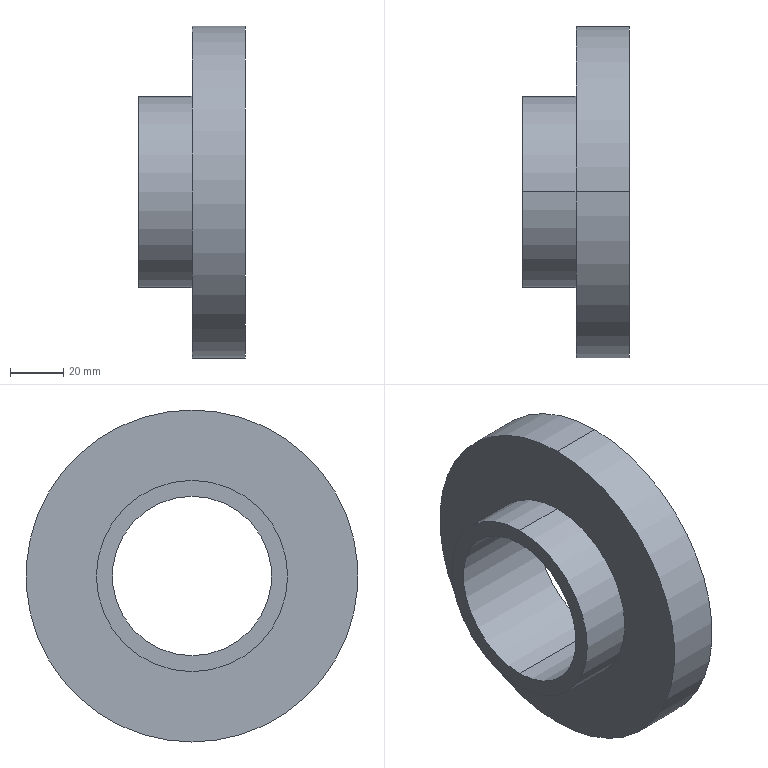Part | SolidWorks | features Revolution 1 | 1 solid | 9 faces | box 40 x 125 x 125 mm | volume 213770 mm3 | cylinder 6 | plane 3 | commonest cylinder face diameters 60 x2 72 x2 125 x2
STEP:
#1=CARTESIAN_POINT('',(40.,0.,62.5));
#2=VERTEX_POINT('',#1);
#3=CARTESIAN_POINT('',(40.,0.,-62.5));
#4=VERTEX_POINT('',#3);
#5=CARTESIAN_POINT('',(40.,0.,0.));
#6=DIRECTION('',(-1.,0.,0.));
#7=DIRECTION('',(0.,0.,1.));
#8=AXIS2_PLACEMENT_3D('',#5,#6,#7);
#9=CIRCLE('',#8,62.5);
#10=EDGE_CURVE('',#2,#4,#9,.T.);
#11=ORIENTED_EDGE('',*,*,#10,.T.);
#12=CARTESIAN_POINT('',(20.,0.,-62.5));
#13=VERTEX_POINT('',#12);
#14=CARTESIAN_POINT('',(0.,0.,-62.5));
#15=DIRECTION('',(-1.,0.,0.));
#16=VECTOR('',#15,1000.);
#17=LINE('',#14,#16);
#18=EDGE_CURVE('',#4,#13,#17,.T.);
#19=ORIENTED_EDGE('',*,*,#18,.T.);
#20=CARTESIAN_POINT('',(20.,0.,62.5));
#21=VERTEX_POINT('',#20);
#22=CARTESIAN_POINT('',(20.,0.,0.));
#23=DIRECTION('',(-1.,0.,0.));
#24=DIRECTION('',(0.,0.,1.));
#25=AXIS2_PLACEMENT_3D('',#22,#23,#24);
#26=CIRCLE('',#25,62.5);
#27=EDGE_CURVE('',#21,#13,#26,.T.);
#28=ORIENTED_EDGE('',*,*,#27,.F.);
#29=CARTESIAN_POINT('',(0.,0.,62.5));
#30=DIRECTION('',(-1.,0.,0.));
#31=VECTOR('',#30,1000.);
#32=LINE('',#29,#31);
#33=EDGE_CURVE('',#2,#21,#32,.T.);
#34=ORIENTED_EDGE('',*,*,#33,.F.);
#35=EDGE_LOOP('',(#11,#19,#28,#34));
#36=FACE_OUTER_BOUND('',#35,.T.);
#37=CARTESIAN_POINT('',(0.,0.,0.));
#38=DIRECTION('',(-1.,0.,0.));
#39=DIRECTION('',(0.,0.,1.));
#40=AXIS2_PLACEMENT_3D('',#37,#38,#39);
#41=CYLINDRICAL_SURFACE('',#40,62.5);
#42=ADVANCED_FACE('',(#36),#41,.T.);
#43=CARTESIAN_POINT('',(20.,0.,36.));
#44=VERTEX_POINT('',#43);
#45=CARTESIAN_POINT('',(20.,0.,-36.));
#46=VERTEX_POINT('',#45);
#47=CARTESIAN_POINT('',(20.,0.,0.));
#48=DIRECTION('',(-1.,0.,0.));
#49=DIRECTION('',(0.,0.,1.));
#50=AXIS2_PLACEMENT_3D('',#47,#48,#49);
#51=CIRCLE('',#50,36.);
#52=EDGE_CURVE('',#44,#46,#51,.T.);
#53=ORIENTED_EDGE('',*,*,#52,.T.);
#54=CARTESIAN_POINT('',(0.,0.,-36.));
#55=VERTEX_POINT('',#54);
#56=CARTESIAN_POINT('',(0.,0.,-36.));
#57=DIRECTION('',(-1.,0.,0.));
#58=VECTOR('',#57,1000.);
#59=LINE('',#56,#58);
#60=EDGE_CURVE('',#46,#55,#59,.T.);
#61=ORIENTED_EDGE('',*,*,#60,.T.);
#62=CARTESIAN_POINT('',(0.,0.,36.));
#63=VERTEX_POINT('',#62);
#64=CARTESIAN_POINT('',(0.,0.,0.));
#65=DIRECTION('',(-1.,0.,0.));
#66=DIRECTION('',(0.,0.,1.));
#67=AXIS2_PLACEMENT_3D('',#64,#65,#66);
#68=CIRCLE('',#67,36.);
#69=EDGE_CURVE('',#63,#55,#68,.T.);
#70=ORIENTED_EDGE('',*,*,#69,.F.);
#71=CARTESIAN_POINT('',(0.,0.,36.));
#72=DIRECTION('',(-1.,0.,0.));
#73=VECTOR('',#72,1000.);
#74=LINE('',#71,#73);
#75=EDGE_CURVE('',#44,#63,#74,.T.);
#76=ORIENTED_EDGE('',*,*,#75,.F.);
#77=EDGE_LOOP('',(#53,#61,#70,#76));
#78=FACE_OUTER_BOUND('',#77,.T.);
#79=CARTESIAN_POINT('',(0.,0.,0.));
#80=DIRECTION('',(-1.,0.,0.));
#81=DIRECTION('',(0.,0.,1.));
#82=AXIS2_PLACEMENT_3D('',#79,#80,#81);
#83=CYLINDRICAL_SURFACE('',#82,36.);
#84=ADVANCED_FACE('',(#78),#83,.T.);
#85=CARTESIAN_POINT('',(40.,0.,-30.));
#86=VERTEX_POINT('',#85);
#87=CARTESIAN_POINT('',(40.,0.,30.));
#88=VERTEX_POINT('',#87);
#89=CARTESIAN_POINT('',(40.,0.,0.));
#90=DIRECTION('',(-1.,0.,0.));
#91=DIRECTION('',(0.,0.,1.));
#92=AXIS2_PLACEMENT_3D('',#89,#90,#91);
#93=CIRCLE('',#92,30.);
#94=EDGE_CURVE('',#86,#88,#93,.T.);
#95=ORIENTED_EDGE('',*,*,#94,.F.);
#96=CARTESIAN_POINT('',(0.,0.,-30.));
#97=VERTEX_POINT('',#96);
#98=CARTESIAN_POINT('',(0.,0.,-30.));
#99=DIRECTION('',(-1.,0.,0.));
#100=VECTOR('',#99,1000.);
#101=LINE('',#98,#100);
#102=EDGE_CURVE('',#86,#97,#101,.T.);
#103=ORIENTED_EDGE('',*,*,#102,.T.);
#104=CARTESIAN_POINT('',(0.,0.,30.));
#105=VERTEX_POINT('',#104);
#106=CARTESIAN_POINT('',(0.,0.,0.));
#107=DIRECTION('',(-1.,0.,0.));
#108=DIRECTION('',(0.,0.,1.));
#109=AXIS2_PLACEMENT_3D('',#106,#107,#108);
#110=CIRCLE('',#109,30.);
#111=EDGE_CURVE('',#97,#105,#110,.T.);
#112=ORIENTED_EDGE('',*,*,#111,.T.);
#113=CARTESIAN_POINT('',(0.,0.,30.));
#114=DIRECTION('',(-1.,0.,0.));
#115=VECTOR('',#114,1000.);
#116=LINE('',#113,#115);
#117=EDGE_CURVE('',#88,#105,#116,.T.);
#118=ORIENTED_EDGE('',*,*,#117,.F.);
#119=EDGE_LOOP('',(#95,#103,#112,#118));
#120=FACE_OUTER_BOUND('',#119,.T.);
#121=CARTESIAN_POINT('',(0.,0.,0.));
#122=DIRECTION('',(-1.,0.,0.));
#123=DIRECTION('',(0.,0.,1.));
#124=AXIS2_PLACEMENT_3D('',#121,#122,#123);
#125=CYLINDRICAL_SURFACE('',#124,30.);
#126=ADVANCED_FACE('',(#120),#125,.F.);
#127=ORIENTED_EDGE('',*,*,#102,.F.);
#128=CARTESIAN_POINT('',(40.,0.,0.));
#129=DIRECTION('',(-1.,0.,0.));
#130=DIRECTION('',(0.,0.,1.));
#131=AXIS2_PLACEMENT_3D('',#128,#129,#130);
#132=CIRCLE('',#131,30.);
#133=EDGE_CURVE('',#88,#86,#132,.T.);
#134=ORIENTED_EDGE('',*,*,#133,.F.);
#135=ORIENTED_EDGE('',*,*,#117,.T.);
#136=CARTESIAN_POINT('',(0.,0.,0.));
#137=DIRECTION('',(-1.,0.,0.));
#138=DIRECTION('',(0.,0.,1.));
#139=AXIS2_PLACEMENT_3D('',#136,#137,#138);
#140=CIRCLE('',#139,30.);
#141=EDGE_CURVE('',#105,#97,#140,.T.);
#142=ORIENTED_EDGE('',*,*,#141,.T.);
#143=EDGE_LOOP('',(#127,#134,#135,#142));
#144=FACE_OUTER_BOUND('',#143,.T.);
#145=CARTESIAN_POINT('',(0.,0.,0.));
#146=DIRECTION('',(-1.,0.,0.));
#147=DIRECTION('',(0.,0.,1.));
#148=AXIS2_PLACEMENT_3D('',#145,#146,#147);
#149=CYLINDRICAL_SURFACE('',#148,30.);
#150=ADVANCED_FACE('',(#144),#149,.F.);
#151=ORIENTED_EDGE('',*,*,#69,.T.);
#152=CARTESIAN_POINT('',(0.,0.,0.));
#153=DIRECTION('',(-1.,0.,0.));
#154=DIRECTION('',(0.,0.,1.));
#155=AXIS2_PLACEMENT_3D('',#152,#153,#154);
#156=CIRCLE('',#155,36.);
#157=EDGE_CURVE('',#55,#63,#156,.T.);
#158=ORIENTED_EDGE('',*,*,#157,.T.);
#159=EDGE_LOOP('',(#151,#158));
#160=FACE_OUTER_BOUND('',#159,.T.);
#161=ORIENTED_EDGE('',*,*,#141,.F.);
#162=ORIENTED_EDGE('',*,*,#111,.F.);
#163=EDGE_LOOP('',(#161,#162));
#164=FACE_BOUND('',#163,.T.);
#165=CARTESIAN_POINT('',(0.,-30.,0.));
#166=DIRECTION('',(-1.,0.,0.));
#167=DIRECTION('',(0.,0.,1.));
#168=AXIS2_PLACEMENT_3D('',#165,#166,#167);
#169=PLANE('',#168);
#170=ADVANCED_FACE('',(#160,#164),#169,.T.);
#171=ORIENTED_EDGE('',*,*,#60,.F.);
#172=CARTESIAN_POINT('',(20.,0.,0.));
#173=DIRECTION('',(-1.,0.,0.));
#174=DIRECTION('',(0.,0.,1.));
#175=AXIS2_PLACEMENT_3D('',#172,#173,#174);
#176=CIRCLE('',#175,36.);
#177=EDGE_CURVE('',#46,#44,#176,.T.);
#178=ORIENTED_EDGE('',*,*,#177,.T.);
#179=ORIENTED_EDGE('',*,*,#75,.T.);
#180=ORIENTED_EDGE('',*,*,#157,.F.);
#181=EDGE_LOOP('',(#171,#178,#179,#180));
#182=FACE_OUTER_BOUND('',#181,.T.);
#183=CARTESIAN_POINT('',(0.,0.,0.));
#184=DIRECTION('',(-1.,0.,0.));
#185=DIRECTION('',(0.,0.,1.));
#186=AXIS2_PLACEMENT_3D('',#183,#184,#185);
#187=CYLINDRICAL_SURFACE('',#186,36.);
#188=ADVANCED_FACE('',(#182),#187,.T.);
#189=ORIENTED_EDGE('',*,*,#27,.T.);
#190=CARTESIAN_POINT('',(20.,0.,0.));
#191=DIRECTION('',(-1.,0.,0.));
#192=DIRECTION('',(0.,0.,1.));
#193=AXIS2_PLACEMENT_3D('',#190,#191,#192);
#194=CIRCLE('',#193,62.5);
#195=EDGE_CURVE('',#13,#21,#194,.T.);
#196=ORIENTED_EDGE('',*,*,#195,.T.);
#197=EDGE_LOOP('',(#189,#196));
#198=FACE_OUTER_BOUND('',#197,.T.);
#199=ORIENTED_EDGE('',*,*,#52,.F.);
#200=ORIENTED_EDGE('',*,*,#177,.F.);
#201=EDGE_LOOP('',(#199,#200));
#202=FACE_BOUND('',#201,.T.);
#203=CARTESIAN_POINT('',(20.,-36.,0.));
#204=DIRECTION('',(-1.,0.,0.));
#205=DIRECTION('',(0.,0.,1.));
#206=AXIS2_PLACEMENT_3D('',#203,#204,#205);
#207=PLANE('',#206);
#208=ADVANCED_FACE('',(#198,#202),#207,.T.);
#209=ORIENTED_EDGE('',*,*,#18,.F.);
#210=CARTESIAN_POINT('',(40.,0.,0.));
#211=DIRECTION('',(-1.,0.,0.));
#212=DIRECTION('',(0.,0.,1.));
#213=AXIS2_PLACEMENT_3D('',#210,#211,#212);
#214=CIRCLE('',#213,62.5);
#215=EDGE_CURVE('',#4,#2,#214,.T.);
#216=ORIENTED_EDGE('',*,*,#215,.T.);
#217=ORIENTED_EDGE('',*,*,#33,.T.);
#218=ORIENTED_EDGE('',*,*,#195,.F.);
#219=EDGE_LOOP('',(#209,#216,#217,#218));
#220=FACE_OUTER_BOUND('',#219,.T.);
#221=CARTESIAN_POINT('',(0.,0.,0.));
#222=DIRECTION('',(-1.,0.,0.));
#223=DIRECTION('',(0.,0.,1.));
#224=AXIS2_PLACEMENT_3D('',#221,#222,#223);
#225=CYLINDRICAL_SURFACE('',#224,62.5);
#226=ADVANCED_FACE('',(#220),#225,.T.);
#227=ORIENTED_EDGE('',*,*,#133,.T.);
#228=ORIENTED_EDGE('',*,*,#94,.T.);
#229=EDGE_LOOP('',(#227,#228));
#230=FACE_BOUND('',#229,.T.);
#231=ORIENTED_EDGE('',*,*,#10,.F.);
#232=ORIENTED_EDGE('',*,*,#215,.F.);
#233=EDGE_LOOP('',(#231,#232));
#234=FACE_OUTER_BOUND('',#233,.T.);
#235=CARTESIAN_POINT('',(40.,-62.5,0.));
#236=DIRECTION('',(1.,0.,0.));
#237=DIRECTION('',(0.,0.,-1.));
#238=AXIS2_PLACEMENT_3D('',#235,#236,#237);
#239=PLANE('',#238);
#240=ADVANCED_FACE('',(#230,#234),#239,.T.);
#241=CLOSED_SHELL('',(#42,#84,#126,#150,#170,#188,#208,#226,#240));
#242=MANIFOLD_SOLID_BREP('',#241);
#243=CARTESIAN_POINT('',(0.,0.,0.));
#244=DIRECTION('',(0.,0.,1.));
#245=DIRECTION('',(1.,0.,0.));
#246=AXIS2_PLACEMENT_3D('',#243,#244,#245);
#247=(LENGTH_UNIT()NAMED_UNIT(*)SI_UNIT(.MILLI.,.METRE.));
#248=UNCERTAINTY_MEASURE_WITH_UNIT(LENGTH_MEASURE(0.00001),#247,'','');
#249=(NAMED_UNIT(*)PLANE_ANGLE_UNIT()SI_UNIT($,.RADIAN.));
#250=(NAMED_UNIT(*)SI_UNIT($,.STERADIAN.)SOLID_ANGLE_UNIT());
#251=(GEOMETRIC_REPRESENTATION_CONTEXT(3)GLOBAL_UNCERTAINTY_ASSIGNED_CONTEXT((#248))GLOBAL_UNIT_ASSIGNED_CONTEXT((#247,#249,#250))REPRESENTATION_CONTEXT('',''));
#252=ADVANCED_BREP_SHAPE_REPRESENTATION('',(#242,#246),#251);